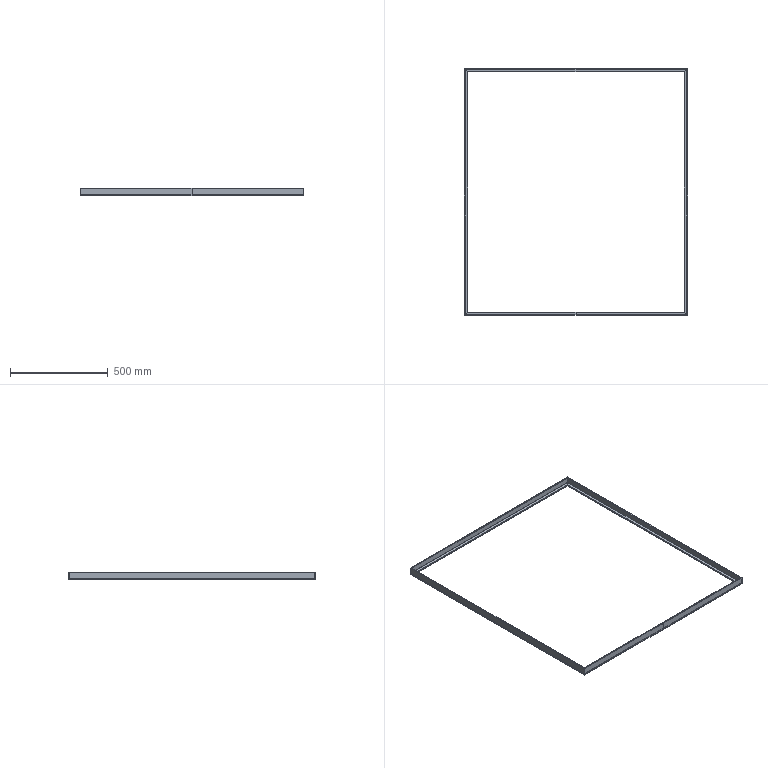Part | SolidWorks | features Sweep 1 | 1 solid | 90 faces | box 1140 x 1260 x 40 mm | volume 435262 mm3 | plane 90